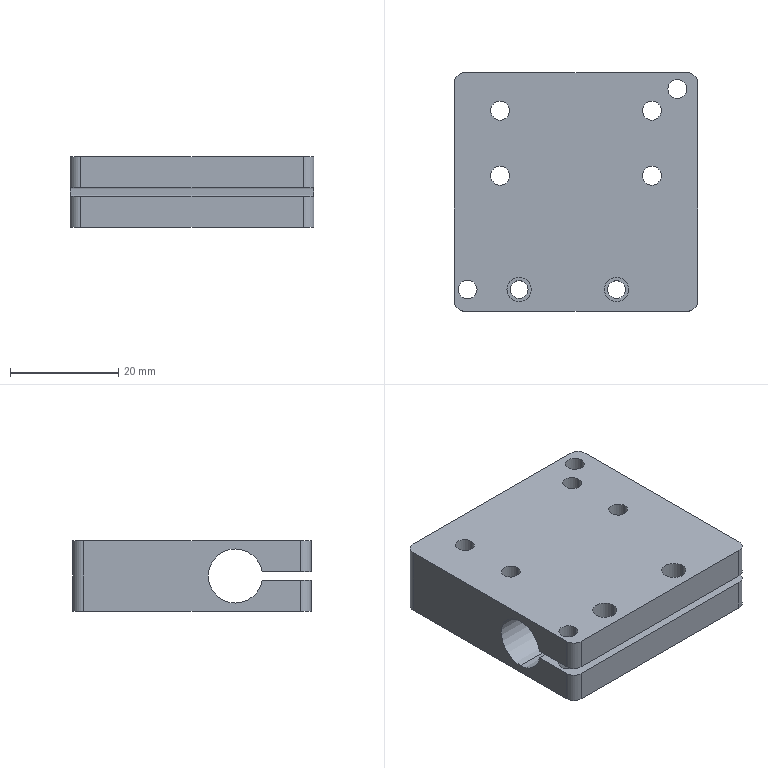Part | STEP file | 1 solid | 40 faces | box 45 x 44 x 13 mm | volume 20538 mm3 | cylinder 31 | plane 9 | commonest cylinder face diameters 3.5 x14 4 x6 3.3 x4 4.5 x4 10 x3